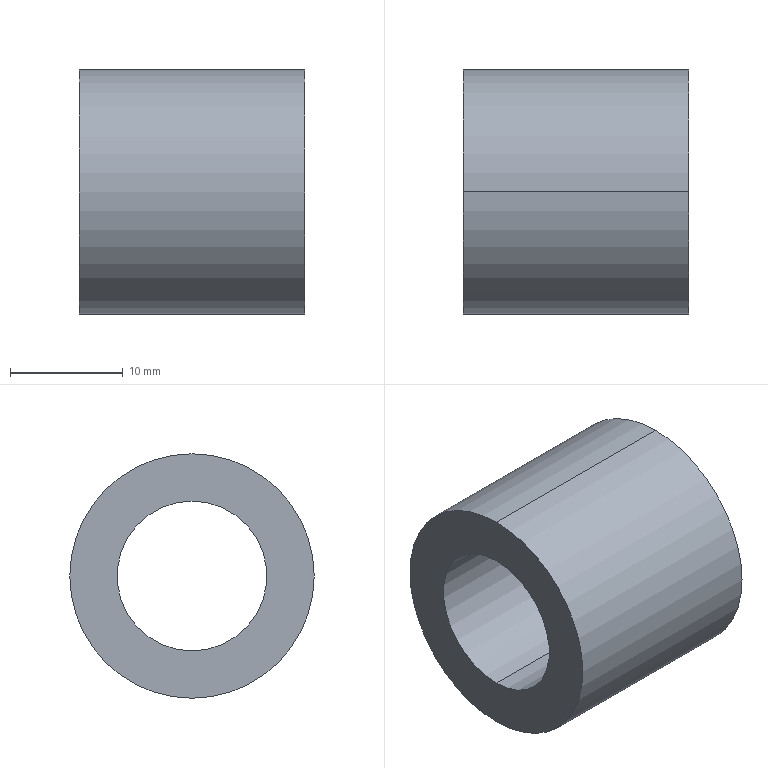Part | SolidWorks | features Extrusion 1 | 1 solid | 6 faces | box 20 x 21.7 x 21.7 mm | volume 4618 mm3 | cylinder 4 | plane 2 | commonest cylinder face diameters 13.3 x2 21.7 x2
STEP:
#1=CARTESIAN_POINT('',(20.,0.,6.65));
#2=VERTEX_POINT('',#1);
#3=CARTESIAN_POINT('',(20.,0.,-6.65));
#4=VERTEX_POINT('',#3);
#5=CARTESIAN_POINT('',(20.,0.,0.));
#6=DIRECTION('',(1.,0.,0.));
#7=DIRECTION('',(0.,0.,-1.));
#8=AXIS2_PLACEMENT_3D('',#5,#6,#7);
#9=CIRCLE('',#8,6.65);
#10=EDGE_CURVE('',#2,#4,#9,.T.);
#11=ORIENTED_EDGE('',*,*,#10,.T.);
#12=CARTESIAN_POINT('',(0.,0.,-6.65));
#13=VERTEX_POINT('',#12);
#14=CARTESIAN_POINT('',(20.,0.,-6.65));
#15=DIRECTION('',(-1.,0.,0.));
#16=VECTOR('',#15,1000.);
#17=LINE('',#14,#16);
#18=EDGE_CURVE('',#4,#13,#17,.T.);
#19=ORIENTED_EDGE('',*,*,#18,.T.);
#20=CARTESIAN_POINT('',(0.,0.,6.65));
#21=VERTEX_POINT('',#20);
#22=CARTESIAN_POINT('',(0.,0.,0.));
#23=DIRECTION('',(1.,0.,0.));
#24=DIRECTION('',(0.,0.,-1.));
#25=AXIS2_PLACEMENT_3D('',#22,#23,#24);
#26=CIRCLE('',#25,6.65);
#27=EDGE_CURVE('',#21,#13,#26,.T.);
#28=ORIENTED_EDGE('',*,*,#27,.F.);
#29=CARTESIAN_POINT('',(20.,0.,6.65));
#30=DIRECTION('',(-1.,0.,0.));
#31=VECTOR('',#30,1000.);
#32=LINE('',#29,#31);
#33=EDGE_CURVE('',#2,#21,#32,.T.);
#34=ORIENTED_EDGE('',*,*,#33,.F.);
#35=EDGE_LOOP('',(#11,#19,#28,#34));
#36=FACE_OUTER_BOUND('',#35,.T.);
#37=CARTESIAN_POINT('',(20.,0.,0.));
#38=DIRECTION('',(-1.,0.,0.));
#39=DIRECTION('',(0.,0.,1.));
#40=AXIS2_PLACEMENT_3D('',#37,#38,#39);
#41=CYLINDRICAL_SURFACE('',#40,6.65);
#42=ADVANCED_FACE('',(#36),#41,.F.);
#43=CARTESIAN_POINT('',(20.,0.,-10.85));
#44=VERTEX_POINT('',#43);
#45=CARTESIAN_POINT('',(20.,0.,10.85));
#46=VERTEX_POINT('',#45);
#47=CARTESIAN_POINT('',(20.,0.,0.));
#48=DIRECTION('',(1.,0.,0.));
#49=DIRECTION('',(0.,0.,-1.));
#50=AXIS2_PLACEMENT_3D('',#47,#48,#49);
#51=CIRCLE('',#50,10.85);
#52=EDGE_CURVE('',#44,#46,#51,.T.);
#53=ORIENTED_EDGE('',*,*,#52,.F.);
#54=CARTESIAN_POINT('',(0.,0.,-10.85));
#55=VERTEX_POINT('',#54);
#56=CARTESIAN_POINT('',(20.,0.,-10.85));
#57=DIRECTION('',(-1.,0.,0.));
#58=VECTOR('',#57,1000.);
#59=LINE('',#56,#58);
#60=EDGE_CURVE('',#44,#55,#59,.T.);
#61=ORIENTED_EDGE('',*,*,#60,.T.);
#62=CARTESIAN_POINT('',(0.,0.,10.85));
#63=VERTEX_POINT('',#62);
#64=CARTESIAN_POINT('',(0.,0.,0.));
#65=DIRECTION('',(1.,0.,0.));
#66=DIRECTION('',(0.,0.,-1.));
#67=AXIS2_PLACEMENT_3D('',#64,#65,#66);
#68=CIRCLE('',#67,10.85);
#69=EDGE_CURVE('',#55,#63,#68,.T.);
#70=ORIENTED_EDGE('',*,*,#69,.T.);
#71=CARTESIAN_POINT('',(20.,0.,10.85));
#72=DIRECTION('',(-1.,0.,0.));
#73=VECTOR('',#72,1000.);
#74=LINE('',#71,#73);
#75=EDGE_CURVE('',#46,#63,#74,.T.);
#76=ORIENTED_EDGE('',*,*,#75,.F.);
#77=EDGE_LOOP('',(#53,#61,#70,#76));
#78=FACE_OUTER_BOUND('',#77,.T.);
#79=CARTESIAN_POINT('',(20.,0.,0.));
#80=DIRECTION('',(-1.,0.,0.));
#81=DIRECTION('',(0.,0.,1.));
#82=AXIS2_PLACEMENT_3D('',#79,#80,#81);
#83=CYLINDRICAL_SURFACE('',#82,10.85);
#84=ADVANCED_FACE('',(#78),#83,.T.);
#85=CARTESIAN_POINT('',(20.,0.,0.));
#86=DIRECTION('',(1.,0.,0.));
#87=DIRECTION('',(0.,0.,-1.));
#88=AXIS2_PLACEMENT_3D('',#85,#86,#87);
#89=CIRCLE('',#88,10.85);
#90=EDGE_CURVE('',#46,#44,#89,.T.);
#91=ORIENTED_EDGE('',*,*,#90,.T.);
#92=ORIENTED_EDGE('',*,*,#52,.T.);
#93=EDGE_LOOP('',(#91,#92));
#94=FACE_OUTER_BOUND('',#93,.T.);
#95=ORIENTED_EDGE('',*,*,#10,.F.);
#96=CARTESIAN_POINT('',(20.,0.,0.));
#97=DIRECTION('',(1.,0.,0.));
#98=DIRECTION('',(0.,0.,-1.));
#99=AXIS2_PLACEMENT_3D('',#96,#97,#98);
#100=CIRCLE('',#99,6.65);
#101=EDGE_CURVE('',#4,#2,#100,.T.);
#102=ORIENTED_EDGE('',*,*,#101,.F.);
#103=EDGE_LOOP('',(#95,#102));
#104=FACE_BOUND('',#103,.T.);
#105=CARTESIAN_POINT('',(20.,0.,0.));
#106=DIRECTION('',(1.,0.,0.));
#107=DIRECTION('',(0.,0.,-1.));
#108=AXIS2_PLACEMENT_3D('',#105,#106,#107);
#109=PLANE('',#108);
#110=ADVANCED_FACE('',(#94,#104),#109,.T.);
#111=CARTESIAN_POINT('',(0.,0.,0.));
#112=DIRECTION('',(1.,0.,0.));
#113=DIRECTION('',(0.,0.,-1.));
#114=AXIS2_PLACEMENT_3D('',#111,#112,#113);
#115=CIRCLE('',#114,10.85);
#116=EDGE_CURVE('',#63,#55,#115,.T.);
#117=ORIENTED_EDGE('',*,*,#116,.F.);
#118=ORIENTED_EDGE('',*,*,#69,.F.);
#119=EDGE_LOOP('',(#117,#118));
#120=FACE_OUTER_BOUND('',#119,.T.);
#121=ORIENTED_EDGE('',*,*,#27,.T.);
#122=CARTESIAN_POINT('',(0.,0.,0.));
#123=DIRECTION('',(1.,0.,0.));
#124=DIRECTION('',(0.,0.,-1.));
#125=AXIS2_PLACEMENT_3D('',#122,#123,#124);
#126=CIRCLE('',#125,6.65);
#127=EDGE_CURVE('',#13,#21,#126,.T.);
#128=ORIENTED_EDGE('',*,*,#127,.T.);
#129=EDGE_LOOP('',(#121,#128));
#130=FACE_BOUND('',#129,.T.);
#131=CARTESIAN_POINT('',(0.,0.,0.));
#132=DIRECTION('',(1.,0.,0.));
#133=DIRECTION('',(0.,0.,-1.));
#134=AXIS2_PLACEMENT_3D('',#131,#132,#133);
#135=PLANE('',#134);
#136=ADVANCED_FACE('',(#120,#130),#135,.F.);
#137=ORIENTED_EDGE('',*,*,#60,.F.);
#138=ORIENTED_EDGE('',*,*,#90,.F.);
#139=ORIENTED_EDGE('',*,*,#75,.T.);
#140=ORIENTED_EDGE('',*,*,#116,.T.);
#141=EDGE_LOOP('',(#137,#138,#139,#140));
#142=FACE_OUTER_BOUND('',#141,.T.);
#143=CARTESIAN_POINT('',(20.,0.,0.));
#144=DIRECTION('',(-1.,0.,0.));
#145=DIRECTION('',(0.,0.,1.));
#146=AXIS2_PLACEMENT_3D('',#143,#144,#145);
#147=CYLINDRICAL_SURFACE('',#146,10.85);
#148=ADVANCED_FACE('',(#142),#147,.T.);
#149=ORIENTED_EDGE('',*,*,#18,.F.);
#150=ORIENTED_EDGE('',*,*,#101,.T.);
#151=ORIENTED_EDGE('',*,*,#33,.T.);
#152=ORIENTED_EDGE('',*,*,#127,.F.);
#153=EDGE_LOOP('',(#149,#150,#151,#152));
#154=FACE_OUTER_BOUND('',#153,.T.);
#155=CARTESIAN_POINT('',(20.,0.,0.));
#156=DIRECTION('',(-1.,0.,0.));
#157=DIRECTION('',(0.,0.,1.));
#158=AXIS2_PLACEMENT_3D('',#155,#156,#157);
#159=CYLINDRICAL_SURFACE('',#158,6.65);
#160=ADVANCED_FACE('',(#154),#159,.F.);
#161=CLOSED_SHELL('',(#42,#84,#110,#136,#148,#160));
#162=MANIFOLD_SOLID_BREP('',#161);
#163=CARTESIAN_POINT('',(0.,0.,0.));
#164=DIRECTION('',(0.,0.,1.));
#165=DIRECTION('',(1.,0.,0.));
#166=AXIS2_PLACEMENT_3D('',#163,#164,#165);
#167=(LENGTH_UNIT()NAMED_UNIT(*)SI_UNIT(.MILLI.,.METRE.));
#168=UNCERTAINTY_MEASURE_WITH_UNIT(LENGTH_MEASURE(0.00001),#167,'','');
#169=(NAMED_UNIT(*)PLANE_ANGLE_UNIT()SI_UNIT($,.RADIAN.));
#170=(NAMED_UNIT(*)SI_UNIT($,.STERADIAN.)SOLID_ANGLE_UNIT());
#171=(GEOMETRIC_REPRESENTATION_CONTEXT(3)GLOBAL_UNCERTAINTY_ASSIGNED_CONTEXT((#168))GLOBAL_UNIT_ASSIGNED_CONTEXT((#167,#169,#170))REPRESENTATION_CONTEXT('',''));
#172=ADVANCED_BREP_SHAPE_REPRESENTATION('',(#162,#166),#171);